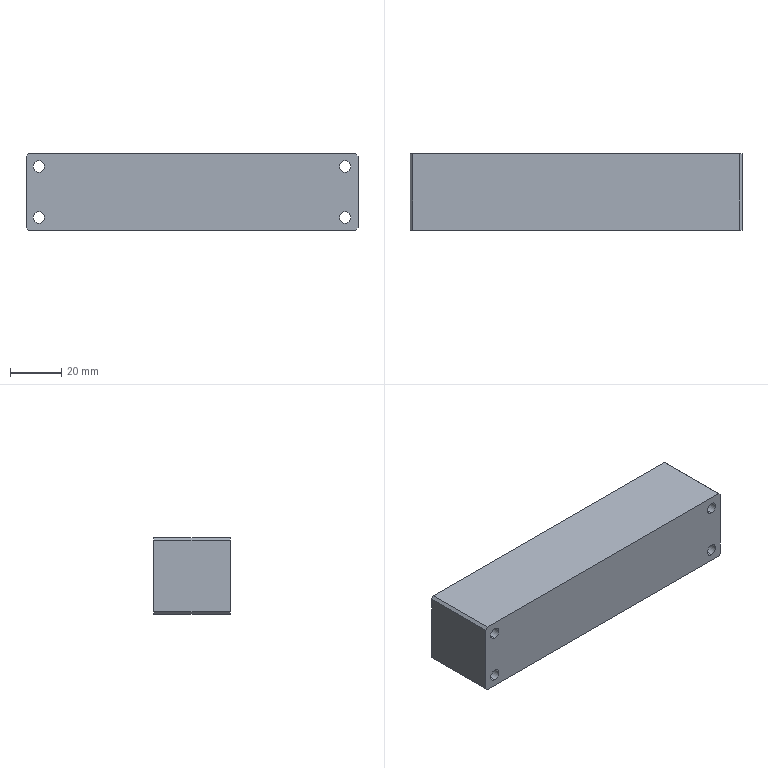Part | SolidWorks | features HoleWzd 3, Chamfer 1, Extrusion 1 | 1 solid | 67 faces | box 130 x 30 x 30 mm | volume 99886 mm3 | cylinder 30 | plane 21 | cone 16 | commonest cylinder face diameters 7.9 x12 4.5 x8 8 x8 10.7 x2